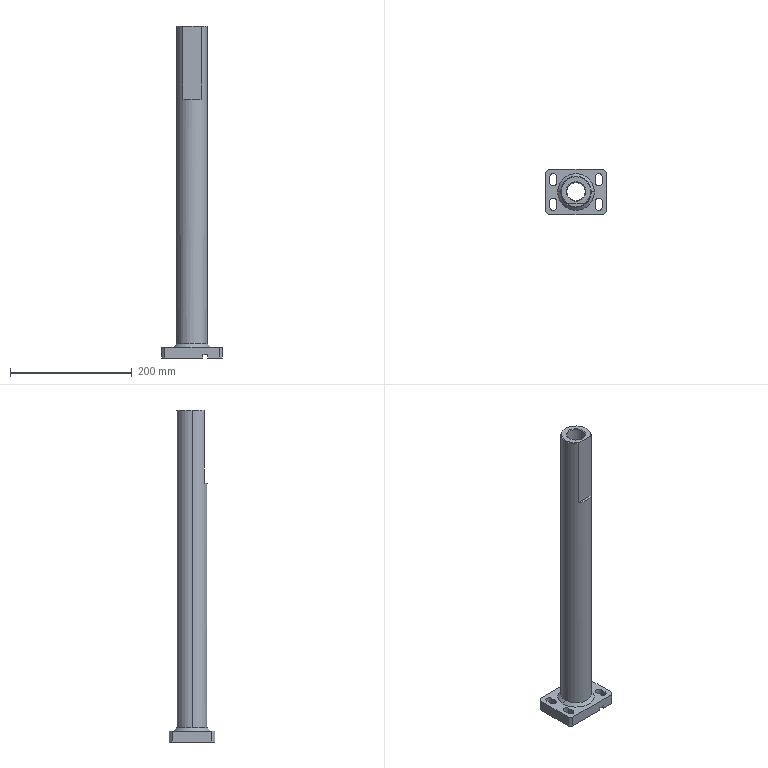Part | STEP file | PN_0041 | 1 solid | 44 faces | box 100 x 75 x 545 mm | volume 756375 mm3 | plane 25 | cylinder 12 | cone 7 | commonest cylinder face diameters 11 x8 30 x2 50 x2